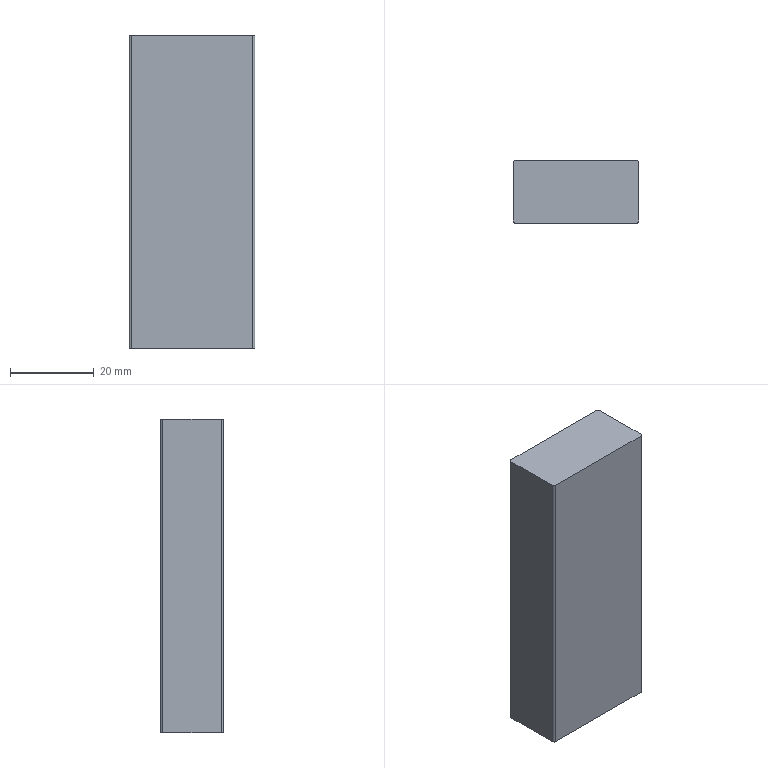Part | STEP file | 1 solid | 13 faces | box 30 x 15 x 75 mm | volume 33035 mm3 | plane 6 | cylinder 5 | cone 2 | commonest cylinder face diameters 1 x4 5 x1
STEP:
#1=CARTESIAN_POINT('',(0.,0.,0.));
#2=DIRECTION('',(0.,0.,1.));
#3=DIRECTION('',(1.,0.,0.));
#4=AXIS2_PLACEMENT_3D('',#1,#2,#3);
#5=CARTESIAN_POINT('',(1735.957,351.98,-43.381));
#6=VERTEX_POINT('',#5);
#7=CARTESIAN_POINT('',(1735.957,337.98,-43.381));
#8=VERTEX_POINT('',#7);
#9=CARTESIAN_POINT('',(1735.957,351.98,-43.381));
#10=DIRECTION('',(0.,-1.,0.));
#11=VECTOR('',#10,1.);
#12=LINE('',#9,#11);
#13=CARTESIAN_POINT('',(1735.957,351.98,33.675));
#14=DIRECTION('',(-1.,0.,0.));
#15=DIRECTION('',(0.,-1.,0.));
#16=AXIS2_PLACEMENT_3D('',#13,#14,#15);
#17=PLANE('',#16);
#18=CARTESIAN_POINT('',(0.,-77.056));
#19=DIRECTION('',(1.,0.));
#20=VECTOR('',#19,1.);
#21=LINE('',#18,#20);
#22=(GEOMETRIC_REPRESENTATION_CONTEXT(2)PARAMETRIC_REPRESENTATION_CONTEXT()REPRESENTATION_CONTEXT('',''));
#23=DEFINITIONAL_REPRESENTATION('',(#21),#22);
#24=PCURVE('',#17,#23);
#25=CARTESIAN_POINT('',(1735.457,337.98,-43.381));
#26=DIRECTION('',(0.,0.,1.));
#27=DIRECTION('',(-1.,0.,0.));
#28=AXIS2_PLACEMENT_3D('',#25,#26,#27);
#29=PLANE('',#28);
#30=CARTESIAN_POINT('',(-0.5,-14.));
#31=DIRECTION('',(0.,1.));
#32=VECTOR('',#31,1.);
#33=LINE('',#30,#32);
#34=(GEOMETRIC_REPRESENTATION_CONTEXT(2)PARAMETRIC_REPRESENTATION_CONTEXT()REPRESENTATION_CONTEXT('',''));
#35=DEFINITIONAL_REPRESENTATION('',(#33),#34);
#36=PCURVE('',#29,#35);
#37=SURFACE_CURVE('',#12,(#24,#36),.PCURVE_S1.);
#38=EDGE_CURVE('',#6,#8,#37,.T.);
#39=ORIENTED_EDGE('',*,*,#38,.F.);
#40=CARTESIAN_POINT('',(1735.957,351.98,31.619));
#41=VERTEX_POINT('',#40);
#42=CARTESIAN_POINT('',(1735.957,351.98,33.675));
#43=DIRECTION('',(0.,0.,-1.));
#44=VECTOR('',#43,1.);
#45=LINE('',#42,#44);
#46=CARTESIAN_POINT('',(0.,0.));
#47=DIRECTION('',(0.,-1.));
#48=VECTOR('',#47,1.);
#49=LINE('',#46,#48);
#50=(GEOMETRIC_REPRESENTATION_CONTEXT(2)PARAMETRIC_REPRESENTATION_CONTEXT()REPRESENTATION_CONTEXT('',''));
#51=DEFINITIONAL_REPRESENTATION('',(#49),#50);
#52=PCURVE('',#17,#51);
#53=CARTESIAN_POINT('',(1735.457,351.98,33.675));
#54=DIRECTION('',(0.,0.,-1.));
#55=DIRECTION('',(1.,0.,0.));
#56=AXIS2_PLACEMENT_3D('',#53,#54,#55);
#57=CYLINDRICAL_SURFACE('',#56,0.5);
#58=CARTESIAN_POINT('',(6.283,0.));
#59=DIRECTION('',(0.,1.));
#60=VECTOR('',#59,1.);
#61=LINE('',#58,#60);
#62=(GEOMETRIC_REPRESENTATION_CONTEXT(2)PARAMETRIC_REPRESENTATION_CONTEXT()REPRESENTATION_CONTEXT('',''));
#63=DEFINITIONAL_REPRESENTATION('',(#61),#62);
#64=PCURVE('',#57,#63);
#65=SURFACE_CURVE('',#45,(#52,#64),.PCURVE_S1.);
#66=EDGE_CURVE('',#41,#6,#65,.T.);
#67=ORIENTED_EDGE('',*,*,#66,.F.);
#68=CARTESIAN_POINT('',(1735.957,337.98,31.619));
#69=VERTEX_POINT('',#68);
#70=CARTESIAN_POINT('',(1735.957,337.98,31.619));
#71=DIRECTION('',(0.,-1.,0.));
#72=VECTOR('',#71,1.);
#73=LINE('',#70,#72);
#74=CARTESIAN_POINT('',(14.,-2.056));
#75=DIRECTION('',(1.,0.));
#76=VECTOR('',#75,1.);
#77=LINE('',#74,#76);
#78=(GEOMETRIC_REPRESENTATION_CONTEXT(2)PARAMETRIC_REPRESENTATION_CONTEXT()REPRESENTATION_CONTEXT('',''));
#79=DEFINITIONAL_REPRESENTATION('',(#77),#78);
#80=PCURVE('',#17,#79);
#81=CARTESIAN_POINT('',(1735.457,337.98,31.619));
#82=DIRECTION('',(0.,0.,1.));
#83=DIRECTION('',(-1.,0.,0.));
#84=AXIS2_PLACEMENT_3D('',#81,#82,#83);
#85=PLANE('',#84);
#86=CARTESIAN_POINT('',(-0.5,0.));
#87=DIRECTION('',(0.,1.));
#88=VECTOR('',#87,1.);
#89=LINE('',#86,#88);
#90=(GEOMETRIC_REPRESENTATION_CONTEXT(2)PARAMETRIC_REPRESENTATION_CONTEXT()REPRESENTATION_CONTEXT('',''));
#91=DEFINITIONAL_REPRESENTATION('',(#89),#90);
#92=PCURVE('',#85,#91);
#93=SURFACE_CURVE('',#73,(#80,#92),.PCURVE_S1.);
#94=EDGE_CURVE('',#41,#69,#93,.T.);
#95=ORIENTED_EDGE('',*,*,#94,.T.);
#96=CARTESIAN_POINT('',(1735.957,337.98,33.675));
#97=DIRECTION('',(0.,0.,-1.));
#98=VECTOR('',#97,1.);
#99=LINE('',#96,#98);
#100=CARTESIAN_POINT('',(14.,0.));
#101=DIRECTION('',(0.,-1.));
#102=VECTOR('',#101,1.);
#103=LINE('',#100,#102);
#104=(GEOMETRIC_REPRESENTATION_CONTEXT(2)PARAMETRIC_REPRESENTATION_CONTEXT()REPRESENTATION_CONTEXT('',''));
#105=DEFINITIONAL_REPRESENTATION('',(#103),#104);
#106=PCURVE('',#17,#105);
#107=CARTESIAN_POINT('',(1735.457,337.98,33.675));
#108=DIRECTION('',(0.,0.,-1.));
#109=DIRECTION('',(1.,0.,0.));
#110=AXIS2_PLACEMENT_3D('',#107,#108,#109);
#111=CYLINDRICAL_SURFACE('',#110,0.5);
#112=CARTESIAN_POINT('',(0.,0.));
#113=DIRECTION('',(0.,1.));
#114=VECTOR('',#113,1.);
#115=LINE('',#112,#114);
#116=(GEOMETRIC_REPRESENTATION_CONTEXT(2)PARAMETRIC_REPRESENTATION_CONTEXT()REPRESENTATION_CONTEXT('',''));
#117=DEFINITIONAL_REPRESENTATION('',(#115),#116);
#118=PCURVE('',#111,#117);
#119=SURFACE_CURVE('',#99,(#106,#118),.PCURVE_S1.);
#120=EDGE_CURVE('',#69,#8,#119,.T.);
#121=ORIENTED_EDGE('',*,*,#120,.T.);
#122=EDGE_LOOP('',(#39,#67,#95,#121));
#123=FACE_BOUND('',#122,.T.);
#124=ADVANCED_FACE('',(#123),#17,.F.);
#125=CARTESIAN_POINT('',(1735.457,337.48,-43.381));
#126=VERTEX_POINT('',#125);
#127=CARTESIAN_POINT('',(1735.457,337.98,-43.381));
#128=DIRECTION('',(0.,0.,-1.));
#129=DIRECTION('',(1.,0.,0.));
#130=AXIS2_PLACEMENT_3D('',#127,#128,#129);
#131=CIRCLE('',#130,0.5);
#132=CARTESIAN_POINT('',(0.,77.056));
#133=DIRECTION('',(1.,0.));
#134=VECTOR('',#133,1.);
#135=LINE('',#132,#134);
#136=(GEOMETRIC_REPRESENTATION_CONTEXT(2)PARAMETRIC_REPRESENTATION_CONTEXT()REPRESENTATION_CONTEXT('',''));
#137=DEFINITIONAL_REPRESENTATION('',(#135),#136);
#138=PCURVE('',#111,#137);
#139=CARTESIAN_POINT('',(-0.5,0.));
#140=CARTESIAN_POINT('',(-0.5,0.866));
#141=CARTESIAN_POINT('',(0.25,0.433));
#142=CARTESIAN_POINT('',(1.,0.));
#143=CARTESIAN_POINT('',(0.25,-0.433));
#144=CARTESIAN_POINT('',(-0.5,-0.866));
#145=CARTESIAN_POINT('',(-0.5,0.));
#146=(BOUNDED_CURVE()B_SPLINE_CURVE(2,(#139,#140,#141,#142,#143,#144,#145),.UNSPECIFIED.,.T.,.F.)B_SPLINE_CURVE_WITH_KNOTS((1,2,2,2,2,1),(-2.094,0.,2.094,4.189,6.283,8.378),.UNSPECIFIED.)CURVE()GEOMETRIC_REPRESENTATION_ITEM()RATIONAL_B_SPLINE_CURVE((1.,0.5,1.,0.5,1.,0.5,1.))REPRESENTATION_ITEM(''));
#147=(GEOMETRIC_REPRESENTATION_CONTEXT(2)PARAMETRIC_REPRESENTATION_CONTEXT()REPRESENTATION_CONTEXT('',''));
#148=DEFINITIONAL_REPRESENTATION('',(#146),#147);
#149=PCURVE('',#29,#148);
#150=SURFACE_CURVE('',#131,(#138,#149),.PCURVE_S1.);
#151=EDGE_CURVE('',#8,#126,#150,.T.);
#152=ORIENTED_EDGE('',*,*,#151,.F.);
#153=ORIENTED_EDGE('',*,*,#120,.F.);
#154=CARTESIAN_POINT('',(1735.457,337.48,31.619));
#155=VERTEX_POINT('',#154);
#156=CARTESIAN_POINT('',(1735.457,337.98,31.619));
#157=DIRECTION('',(0.,0.,-1.));
#158=DIRECTION('',(1.,0.,0.));
#159=AXIS2_PLACEMENT_3D('',#156,#157,#158);
#160=CIRCLE('',#159,0.5);
#161=CARTESIAN_POINT('',(0.,2.056));
#162=DIRECTION('',(1.,0.));
#163=VECTOR('',#162,1.);
#164=LINE('',#161,#163);
#165=(GEOMETRIC_REPRESENTATION_CONTEXT(2)PARAMETRIC_REPRESENTATION_CONTEXT()REPRESENTATION_CONTEXT('',''));
#166=DEFINITIONAL_REPRESENTATION('',(#164),#165);
#167=PCURVE('',#111,#166);
#168=CARTESIAN_POINT('',(-0.5,0.));
#169=CARTESIAN_POINT('',(-0.5,0.866));
#170=CARTESIAN_POINT('',(0.25,0.433));
#171=CARTESIAN_POINT('',(1.,0.));
#172=CARTESIAN_POINT('',(0.25,-0.433));
#173=CARTESIAN_POINT('',(-0.5,-0.866));
#174=CARTESIAN_POINT('',(-0.5,0.));
#175=(BOUNDED_CURVE()B_SPLINE_CURVE(2,(#168,#169,#170,#171,#172,#173,#174),.UNSPECIFIED.,.T.,.F.)B_SPLINE_CURVE_WITH_KNOTS((1,2,2,2,2,1),(-2.094,0.,2.094,4.189,6.283,8.378),.UNSPECIFIED.)CURVE()GEOMETRIC_REPRESENTATION_ITEM()RATIONAL_B_SPLINE_CURVE((1.,0.5,1.,0.5,1.,0.5,1.))REPRESENTATION_ITEM(''));
#176=(GEOMETRIC_REPRESENTATION_CONTEXT(2)PARAMETRIC_REPRESENTATION_CONTEXT()REPRESENTATION_CONTEXT('',''));
#177=DEFINITIONAL_REPRESENTATION('',(#175),#176);
#178=PCURVE('',#85,#177);
#179=SURFACE_CURVE('',#160,(#167,#178),.PCURVE_S1.);
#180=EDGE_CURVE('',#69,#155,#179,.T.);
#181=ORIENTED_EDGE('',*,*,#180,.T.);
#182=CARTESIAN_POINT('',(1735.457,337.48,33.675));
#183=DIRECTION('',(0.,0.,-1.));
#184=VECTOR('',#183,1.);
#185=LINE('',#182,#184);
#186=CARTESIAN_POINT('',(1.571,0.));
#187=DIRECTION('',(0.,1.));
#188=VECTOR('',#187,1.);
#189=LINE('',#186,#188);
#190=(GEOMETRIC_REPRESENTATION_CONTEXT(2)PARAMETRIC_REPRESENTATION_CONTEXT()REPRESENTATION_CONTEXT('',''));
#191=DEFINITIONAL_REPRESENTATION('',(#189),#190);
#192=PCURVE('',#111,#191);
#193=CARTESIAN_POINT('',(1735.457,337.48,33.675));
#194=DIRECTION('',(0.,1.,0.));
#195=DIRECTION('',(0.,0.,-1.));
#196=AXIS2_PLACEMENT_3D('',#193,#194,#195);
#197=PLANE('',#196);
#198=CARTESIAN_POINT('',(0.,0.));
#199=DIRECTION('',(1.,0.));
#200=VECTOR('',#199,1.);
#201=LINE('',#198,#200);
#202=(GEOMETRIC_REPRESENTATION_CONTEXT(2)PARAMETRIC_REPRESENTATION_CONTEXT()REPRESENTATION_CONTEXT('',''));
#203=DEFINITIONAL_REPRESENTATION('',(#201),#202);
#204=PCURVE('',#197,#203);
#205=SURFACE_CURVE('',#185,(#192,#204),.PCURVE_S1.);
#206=EDGE_CURVE('',#155,#126,#205,.T.);
#207=ORIENTED_EDGE('',*,*,#206,.T.);
#208=EDGE_LOOP('',(#152,#153,#181,#207));
#209=FACE_BOUND('',#208,.T.);
#210=ADVANCED_FACE('',(#209),#111,.T.);
#211=CARTESIAN_POINT('',(1706.457,337.48,-43.381));
#212=VERTEX_POINT('',#211);
#213=CARTESIAN_POINT('',(1735.457,337.48,-43.381));
#214=DIRECTION('',(-1.,0.,0.));
#215=VECTOR('',#214,1.);
#216=LINE('',#213,#215);
#217=CARTESIAN_POINT('',(77.056,0.));
#218=DIRECTION('',(0.,1.));
#219=VECTOR('',#218,1.);
#220=LINE('',#217,#219);
#221=(GEOMETRIC_REPRESENTATION_CONTEXT(2)PARAMETRIC_REPRESENTATION_CONTEXT()REPRESENTATION_CONTEXT('',''));
#222=DEFINITIONAL_REPRESENTATION('',(#220),#221);
#223=PCURVE('',#197,#222);
#224=CARTESIAN_POINT('',(0.,0.5));
#225=DIRECTION('',(1.,0.));
#226=VECTOR('',#225,1.);
#227=LINE('',#224,#226);
#228=(GEOMETRIC_REPRESENTATION_CONTEXT(2)PARAMETRIC_REPRESENTATION_CONTEXT()REPRESENTATION_CONTEXT('',''));
#229=DEFINITIONAL_REPRESENTATION('',(#227),#228);
#230=PCURVE('',#29,#229);
#231=SURFACE_CURVE('',#216,(#223,#230),.PCURVE_S1.);
#232=EDGE_CURVE('',#126,#212,#231,.T.);
#233=ORIENTED_EDGE('',*,*,#232,.F.);
#234=ORIENTED_EDGE('',*,*,#206,.F.);
#235=CARTESIAN_POINT('',(1706.457,337.48,31.619));
#236=VERTEX_POINT('',#235);
#237=CARTESIAN_POINT('',(1735.457,337.48,31.619));
#238=DIRECTION('',(-1.,0.,0.));
#239=VECTOR('',#238,1.);
#240=LINE('',#237,#239);
#241=CARTESIAN_POINT('',(2.056,0.));
#242=DIRECTION('',(0.,1.));
#243=VECTOR('',#242,1.);
#244=LINE('',#241,#243);
#245=(GEOMETRIC_REPRESENTATION_CONTEXT(2)PARAMETRIC_REPRESENTATION_CONTEXT()REPRESENTATION_CONTEXT('',''));
#246=DEFINITIONAL_REPRESENTATION('',(#244),#245);
#247=PCURVE('',#197,#246);
#248=CARTESIAN_POINT('',(0.,0.5));
#249=DIRECTION('',(1.,0.));
#250=VECTOR('',#249,1.);
#251=LINE('',#248,#250);
#252=(GEOMETRIC_REPRESENTATION_CONTEXT(2)PARAMETRIC_REPRESENTATION_CONTEXT()REPRESENTATION_CONTEXT('',''));
#253=DEFINITIONAL_REPRESENTATION('',(#251),#252);
#254=PCURVE('',#85,#253);
#255=SURFACE_CURVE('',#240,(#247,#254),.PCURVE_S1.);
#256=EDGE_CURVE('',#155,#236,#255,.T.);
#257=ORIENTED_EDGE('',*,*,#256,.T.);
#258=CARTESIAN_POINT('',(1706.457,337.48,33.675));
#259=DIRECTION('',(0.,0.,-1.));
#260=VECTOR('',#259,1.);
#261=LINE('',#258,#260);
#262=CARTESIAN_POINT('',(0.,29.));
#263=DIRECTION('',(1.,0.));
#264=VECTOR('',#263,1.);
#265=LINE('',#262,#264);
#266=(GEOMETRIC_REPRESENTATION_CONTEXT(2)PARAMETRIC_REPRESENTATION_CONTEXT()REPRESENTATION_CONTEXT('',''));
#267=DEFINITIONAL_REPRESENTATION('',(#265),#266);
#268=PCURVE('',#197,#267);
#269=CARTESIAN_POINT('',(1706.457,337.98,33.675));
#270=DIRECTION('',(0.,0.,-1.));
#271=DIRECTION('',(1.,0.,0.));
#272=AXIS2_PLACEMENT_3D('',#269,#270,#271);
#273=CYLINDRICAL_SURFACE('',#272,0.5);
#274=CARTESIAN_POINT('',(1.571,0.));
#275=DIRECTION('',(0.,1.));
#276=VECTOR('',#275,1.);
#277=LINE('',#274,#276);
#278=(GEOMETRIC_REPRESENTATION_CONTEXT(2)PARAMETRIC_REPRESENTATION_CONTEXT()REPRESENTATION_CONTEXT('',''));
#279=DEFINITIONAL_REPRESENTATION('',(#277),#278);
#280=PCURVE('',#273,#279);
#281=SURFACE_CURVE('',#261,(#268,#280),.PCURVE_S1.);
#282=EDGE_CURVE('',#236,#212,#281,.T.);
#283=ORIENTED_EDGE('',*,*,#282,.T.);
#284=EDGE_LOOP('',(#233,#234,#257,#283));
#285=FACE_BOUND('',#284,.T.);
#286=ADVANCED_FACE('',(#285),#197,.F.);
#287=CARTESIAN_POINT('',(1705.957,337.98,-43.381));
#288=VERTEX_POINT('',#287);
#289=CARTESIAN_POINT('',(1706.457,337.98,-43.381));
#290=DIRECTION('',(0.,0.,-1.));
#291=DIRECTION('',(1.,0.,0.));
#292=AXIS2_PLACEMENT_3D('',#289,#290,#291);
#293=CIRCLE('',#292,0.5);
#294=CARTESIAN_POINT('',(0.,77.056));
#295=DIRECTION('',(1.,0.));
#296=VECTOR('',#295,1.);
#297=LINE('',#294,#296);
#298=(GEOMETRIC_REPRESENTATION_CONTEXT(2)PARAMETRIC_REPRESENTATION_CONTEXT()REPRESENTATION_CONTEXT('',''));
#299=DEFINITIONAL_REPRESENTATION('',(#297),#298);
#300=PCURVE('',#273,#299);
#301=CARTESIAN_POINT('',(28.5,0.));
#302=CARTESIAN_POINT('',(28.5,0.866));
#303=CARTESIAN_POINT('',(29.25,0.433));
#304=CARTESIAN_POINT('',(30.,0.));
#305=CARTESIAN_POINT('',(29.25,-0.433));
#306=CARTESIAN_POINT('',(28.5,-0.866));
#307=CARTESIAN_POINT('',(28.5,0.));
#308=(BOUNDED_CURVE()B_SPLINE_CURVE(2,(#301,#302,#303,#304,#305,#306,#307),.UNSPECIFIED.,.T.,.F.)B_SPLINE_CURVE_WITH_KNOTS((1,2,2,2,2,1),(-2.094,0.,2.094,4.189,6.283,8.378),.UNSPECIFIED.)CURVE()GEOMETRIC_REPRESENTATION_ITEM()RATIONAL_B_SPLINE_CURVE((1.,0.5,1.,0.5,1.,0.5,1.))REPRESENTATION_ITEM(''));
#309=(GEOMETRIC_REPRESENTATION_CONTEXT(2)PARAMETRIC_REPRESENTATION_CONTEXT()REPRESENTATION_CONTEXT('',''));
#310=DEFINITIONAL_REPRESENTATION('',(#308),#309);
#311=PCURVE('',#29,#310);
#312=SURFACE_CURVE('',#293,(#300,#311),.PCURVE_S1.);
#313=EDGE_CURVE('',#212,#288,#312,.T.);
#314=ORIENTED_EDGE('',*,*,#313,.F.);
#315=ORIENTED_EDGE('',*,*,#282,.F.);
#316=CARTESIAN_POINT('',(1705.957,337.98,31.619));
#317=VERTEX_POINT('',#316);
#318=CARTESIAN_POINT('',(1706.457,337.98,31.619));
#319=DIRECTION('',(0.,0.,-1.));
#320=DIRECTION('',(1.,0.,0.));
#321=AXIS2_PLACEMENT_3D('',#318,#319,#320);
#322=CIRCLE('',#321,0.5);
#323=CARTESIAN_POINT('',(0.,2.056));
#324=DIRECTION('',(1.,0.));
#325=VECTOR('',#324,1.);
#326=LINE('',#323,#325);
#327=(GEOMETRIC_REPRESENTATION_CONTEXT(2)PARAMETRIC_REPRESENTATION_CONTEXT()REPRESENTATION_CONTEXT('',''));
#328=DEFINITIONAL_REPRESENTATION('',(#326),#327);
#329=PCURVE('',#273,#328);
#330=CARTESIAN_POINT('',(28.5,0.));
#331=CARTESIAN_POINT('',(28.5,0.866));
#332=CARTESIAN_POINT('',(29.25,0.433));
#333=CARTESIAN_POINT('',(30.,0.));
#334=CARTESIAN_POINT('',(29.25,-0.433));
#335=CARTESIAN_POINT('',(28.5,-0.866));
#336=CARTESIAN_POINT('',(28.5,0.));
#337=(BOUNDED_CURVE()B_SPLINE_CURVE(2,(#330,#331,#332,#333,#334,#335,#336),.UNSPECIFIED.,.T.,.F.)B_SPLINE_CURVE_WITH_KNOTS((1,2,2,2,2,1),(-2.094,0.,2.094,4.189,6.283,8.378),.UNSPECIFIED.)CURVE()GEOMETRIC_REPRESENTATION_ITEM()RATIONAL_B_SPLINE_CURVE((1.,0.5,1.,0.5,1.,0.5,1.))REPRESENTATION_ITEM(''));
#338=(GEOMETRIC_REPRESENTATION_CONTEXT(2)PARAMETRIC_REPRESENTATION_CONTEXT()REPRESENTATION_CONTEXT('',''));
#339=DEFINITIONAL_REPRESENTATION('',(#337),#338);
#340=PCURVE('',#85,#339);
#341=SURFACE_CURVE('',#322,(#329,#340),.PCURVE_S1.);
#342=EDGE_CURVE('',#236,#317,#341,.T.);
#343=ORIENTED_EDGE('',*,*,#342,.T.);
#344=CARTESIAN_POINT('',(1705.957,337.98,33.675));
#345=DIRECTION('',(0.,0.,-1.));
#346=VECTOR('',#345,1.);
#347=LINE('',#344,#346);
#348=CARTESIAN_POINT('',(3.142,0.));
#349=DIRECTION('',(0.,1.));
#350=VECTOR('',#349,1.);
#351=LINE('',#348,#350);
#352=(GEOMETRIC_REPRESENTATION_CONTEXT(2)PARAMETRIC_REPRESENTATION_CONTEXT()REPRESENTATION_CONTEXT('',''));
#353=DEFINITIONAL_REPRESENTATION('',(#351),#352);
#354=PCURVE('',#273,#353);
#355=CARTESIAN_POINT('',(1705.957,337.98,33.675));
#356=DIRECTION('',(1.,0.,0.));
#357=DIRECTION('',(0.,0.,1.));
#358=AXIS2_PLACEMENT_3D('',#355,#356,#357);
#359=PLANE('',#358);
#360=CARTESIAN_POINT('',(0.,0.));
#361=DIRECTION('',(-1.,0.));
#362=VECTOR('',#361,1.);
#363=LINE('',#360,#362);
#364=(GEOMETRIC_REPRESENTATION_CONTEXT(2)PARAMETRIC_REPRESENTATION_CONTEXT()REPRESENTATION_CONTEXT('',''));
#365=DEFINITIONAL_REPRESENTATION('',(#363),#364);
#366=PCURVE('',#359,#365);
#367=SURFACE_CURVE('',#347,(#354,#366),.PCURVE_S1.);
#368=EDGE_CURVE('',#317,#288,#367,.T.);
#369=ORIENTED_EDGE('',*,*,#368,.T.);
#370=EDGE_LOOP('',(#314,#315,#343,#369));
#371=FACE_BOUND('',#370,.T.);
#372=ADVANCED_FACE('',(#371),#273,.T.);
#373=CARTESIAN_POINT('',(1705.957,351.98,-43.381));
#374=VERTEX_POINT('',#373);
#375=CARTESIAN_POINT('',(1705.957,337.98,-43.381));
#376=DIRECTION('',(0.,1.,0.));
#377=VECTOR('',#376,1.);
#378=LINE('',#375,#377);
#379=CARTESIAN_POINT('',(-77.056,0.));
#380=DIRECTION('',(0.,-1.));
#381=VECTOR('',#380,1.);
#382=LINE('',#379,#381);
#383=(GEOMETRIC_REPRESENTATION_CONTEXT(2)PARAMETRIC_REPRESENTATION_CONTEXT()REPRESENTATION_CONTEXT('',''));
#384=DEFINITIONAL_REPRESENTATION('',(#382),#383);
#385=PCURVE('',#359,#384);
#386=CARTESIAN_POINT('',(29.5,0.));
#387=DIRECTION('',(0.,-1.));
#388=VECTOR('',#387,1.);
#389=LINE('',#386,#388);
#390=(GEOMETRIC_REPRESENTATION_CONTEXT(2)PARAMETRIC_REPRESENTATION_CONTEXT()REPRESENTATION_CONTEXT('',''));
#391=DEFINITIONAL_REPRESENTATION('',(#389),#390);
#392=PCURVE('',#29,#391);
#393=SURFACE_CURVE('',#378,(#385,#392),.PCURVE_S1.);
#394=EDGE_CURVE('',#288,#374,#393,.T.);
#395=ORIENTED_EDGE('',*,*,#394,.F.);
#396=ORIENTED_EDGE('',*,*,#368,.F.);
#397=CARTESIAN_POINT('',(1705.957,351.98,31.619));
#398=VERTEX_POINT('',#397);
#399=CARTESIAN_POINT('',(1705.957,337.98,31.619));
#400=DIRECTION('',(0.,1.,0.));
#401=VECTOR('',#400,1.);
#402=LINE('',#399,#401);
#403=CARTESIAN_POINT('',(-2.056,0.));
#404=DIRECTION('',(0.,-1.));
#405=VECTOR('',#404,1.);
#406=LINE('',#403,#405);
#407=(GEOMETRIC_REPRESENTATION_CONTEXT(2)PARAMETRIC_REPRESENTATION_CONTEXT()REPRESENTATION_CONTEXT('',''));
#408=DEFINITIONAL_REPRESENTATION('',(#406),#407);
#409=PCURVE('',#359,#408);
#410=CARTESIAN_POINT('',(29.5,0.));
#411=DIRECTION('',(0.,-1.));
#412=VECTOR('',#411,1.);
#413=LINE('',#410,#412);
#414=(GEOMETRIC_REPRESENTATION_CONTEXT(2)PARAMETRIC_REPRESENTATION_CONTEXT()REPRESENTATION_CONTEXT('',''));
#415=DEFINITIONAL_REPRESENTATION('',(#413),#414);
#416=PCURVE('',#85,#415);
#417=SURFACE_CURVE('',#402,(#409,#416),.PCURVE_S1.);
#418=EDGE_CURVE('',#317,#398,#417,.T.);
#419=ORIENTED_EDGE('',*,*,#418,.T.);
#420=CARTESIAN_POINT('',(1705.957,351.98,33.675));
#421=DIRECTION('',(0.,0.,-1.));
#422=VECTOR('',#421,1.);
#423=LINE('',#420,#422);
#424=CARTESIAN_POINT('',(0.,-14.));
#425=DIRECTION('',(-1.,0.));
#426=VECTOR('',#425,1.);
#427=LINE('',#424,#426);
#428=(GEOMETRIC_REPRESENTATION_CONTEXT(2)PARAMETRIC_REPRESENTATION_CONTEXT()REPRESENTATION_CONTEXT('',''));
#429=DEFINITIONAL_REPRESENTATION('',(#427),#428);
#430=PCURVE('',#359,#429);
#431=CARTESIAN_POINT('',(1706.457,351.98,33.675));
#432=DIRECTION('',(0.,0.,-1.));
#433=DIRECTION('',(1.,0.,0.));
#434=AXIS2_PLACEMENT_3D('',#431,#432,#433);
#435=CYLINDRICAL_SURFACE('',#434,0.5);
#436=CARTESIAN_POINT('',(3.142,0.));
#437=DIRECTION('',(0.,1.));
#438=VECTOR('',#437,1.);
#439=LINE('',#436,#438);
#440=(GEOMETRIC_REPRESENTATION_CONTEXT(2)PARAMETRIC_REPRESENTATION_CONTEXT()REPRESENTATION_CONTEXT('',''));
#441=DEFINITIONAL_REPRESENTATION('',(#439),#440);
#442=PCURVE('',#435,#441);
#443=SURFACE_CURVE('',#423,(#430,#442),.PCURVE_S1.);
#444=EDGE_CURVE('',#398,#374,#443,.T.);
#445=ORIENTED_EDGE('',*,*,#444,.T.);
#446=EDGE_LOOP('',(#395,#396,#419,#445));
#447=FACE_BOUND('',#446,.T.);
#448=ADVANCED_FACE('',(#447),#359,.F.);
#449=CARTESIAN_POINT('',(1706.457,352.48,-43.381));
#450=VERTEX_POINT('',#449);
#451=CARTESIAN_POINT('',(1706.457,351.98,-43.381));
#452=DIRECTION('',(0.,0.,-1.));
#453=DIRECTION('',(1.,0.,0.));
#454=AXIS2_PLACEMENT_3D('',#451,#452,#453);
#455=CIRCLE('',#454,0.5);
#456=CARTESIAN_POINT('',(0.,77.056));
#457=DIRECTION('',(1.,0.));
#458=VECTOR('',#457,1.);
#459=LINE('',#456,#458);
#460=(GEOMETRIC_REPRESENTATION_CONTEXT(2)PARAMETRIC_REPRESENTATION_CONTEXT()REPRESENTATION_CONTEXT('',''));
#461=DEFINITIONAL_REPRESENTATION('',(#459),#460);
#462=PCURVE('',#435,#461);
#463=CARTESIAN_POINT('',(28.5,-14.));
#464=CARTESIAN_POINT('',(28.5,-13.134));
#465=CARTESIAN_POINT('',(29.25,-13.567));
#466=CARTESIAN_POINT('',(30.,-14.));
#467=CARTESIAN_POINT('',(29.25,-14.433));
#468=CARTESIAN_POINT('',(28.5,-14.866));
#469=CARTESIAN_POINT('',(28.5,-14.));
#470=(BOUNDED_CURVE()B_SPLINE_CURVE(2,(#463,#464,#465,#466,#467,#468,#469),.UNSPECIFIED.,.T.,.F.)B_SPLINE_CURVE_WITH_KNOTS((1,2,2,2,2,1),(-2.094,0.,2.094,4.189,6.283,8.378),.UNSPECIFIED.)CURVE()GEOMETRIC_REPRESENTATION_ITEM()RATIONAL_B_SPLINE_CURVE((1.,0.5,1.,0.5,1.,0.5,1.))REPRESENTATION_ITEM(''));
#471=(GEOMETRIC_REPRESENTATION_CONTEXT(2)PARAMETRIC_REPRESENTATION_CONTEXT()REPRESENTATION_CONTEXT('',''));
#472=DEFINITIONAL_REPRESENTATION('',(#470),#471);
#473=PCURVE('',#29,#472);
#474=SURFACE_CURVE('',#455,(#462,#473),.PCURVE_S1.);
#475=EDGE_CURVE('',#374,#450,#474,.T.);
#476=ORIENTED_EDGE('',*,*,#475,.F.);
#477=ORIENTED_EDGE('',*,*,#444,.F.);
#478=CARTESIAN_POINT('',(1706.457,352.48,31.619));
#479=VERTEX_POINT('',#478);
#480=CARTESIAN_POINT('',(1706.457,351.98,31.619));
#481=DIRECTION('',(0.,0.,-1.));
#482=DIRECTION('',(1.,0.,0.));
#483=AXIS2_PLACEMENT_3D('',#480,#481,#482);
#484=CIRCLE('',#483,0.5);
#485=CARTESIAN_POINT('',(0.,2.056));
#486=DIRECTION('',(1.,0.));
#487=VECTOR('',#486,1.);
#488=LINE('',#485,#487);
#489=(GEOMETRIC_REPRESENTATION_CONTEXT(2)PARAMETRIC_REPRESENTATION_CONTEXT()REPRESENTATION_CONTEXT('',''));
#490=DEFINITIONAL_REPRESENTATION('',(#488),#489);
#491=PCURVE('',#435,#490);
#492=CARTESIAN_POINT('',(28.5,-14.));
#493=CARTESIAN_POINT('',(28.5,-13.134));
#494=CARTESIAN_POINT('',(29.25,-13.567));
#495=CARTESIAN_POINT('',(30.,-14.));
#496=CARTESIAN_POINT('',(29.25,-14.433));
#497=CARTESIAN_POINT('',(28.5,-14.866));
#498=CARTESIAN_POINT('',(28.5,-14.));
#499=(BOUNDED_CURVE()B_SPLINE_CURVE(2,(#492,#493,#494,#495,#496,#497,#498),.UNSPECIFIED.,.T.,.F.)B_SPLINE_CURVE_WITH_KNOTS((1,2,2,2,2,1),(-2.094,0.,2.094,4.189,6.283,8.378),.UNSPECIFIED.)CURVE()GEOMETRIC_REPRESENTATION_ITEM()RATIONAL_B_SPLINE_CURVE((1.,0.5,1.,0.5,1.,0.5,1.))REPRESENTATION_ITEM(''));
#500=(GEOMETRIC_REPRESENTATION_CONTEXT(2)PARAMETRIC_REPRESENTATION_CONTEXT()REPRESENTATION_CONTEXT('',''));
#501=DEFINITIONAL_REPRESENTATION('',(#499),#500);
#502=PCURVE('',#85,#501);
#503=SURFACE_CURVE('',#484,(#491,#502),.PCURVE_S1.);
#504=EDGE_CURVE('',#398,#479,#503,.T.);
#505=ORIENTED_EDGE('',*,*,#504,.T.);
#506=CARTESIAN_POINT('',(1706.457,352.48,33.675));
#507=DIRECTION('',(0.,0.,-1.));
#508=VECTOR('',#507,1.);
#509=LINE('',#506,#508);
#510=CARTESIAN_POINT('',(4.712,0.));
#511=DIRECTION('',(0.,1.));
#512=VECTOR('',#511,1.);
#513=LINE('',#510,#512);
#514=(GEOMETRIC_REPRESENTATION_CONTEXT(2)PARAMETRIC_REPRESENTATION_CONTEXT()REPRESENTATION_CONTEXT('',''));
#515=DEFINITIONAL_REPRESENTATION('',(#513),#514);
#516=PCURVE('',#435,#515);
#517=CARTESIAN_POINT('',(1706.457,352.48,33.675));
#518=DIRECTION('',(0.,-1.,0.));
#519=DIRECTION('',(0.,0.,1.));
#520=AXIS2_PLACEMENT_3D('',#517,#518,#519);
#521=PLANE('',#520);
#522=CARTESIAN_POINT('',(0.,0.));
#523=DIRECTION('',(-1.,0.));
#524=VECTOR('',#523,1.);
#525=LINE('',#522,#524);
#526=(GEOMETRIC_REPRESENTATION_CONTEXT(2)PARAMETRIC_REPRESENTATION_CONTEXT()REPRESENTATION_CONTEXT('',''));
#527=DEFINITIONAL_REPRESENTATION('',(#525),#526);
#528=PCURVE('',#521,#527);
#529=SURFACE_CURVE('',#509,(#516,#528),.PCURVE_S1.);
#530=EDGE_CURVE('',#479,#450,#529,.T.);
#531=ORIENTED_EDGE('',*,*,#530,.T.);
#532=EDGE_LOOP('',(#476,#477,#505,#531));
#533=FACE_BOUND('',#532,.T.);
#534=ADVANCED_FACE('',(#533),#435,.T.);
#535=CARTESIAN_POINT('',(1735.457,352.48,-43.381));
#536=VERTEX_POINT('',#535);
#537=CARTESIAN_POINT('',(1706.457,352.48,-43.381));
#538=DIRECTION('',(1.,0.,0.));
#539=VECTOR('',#538,1.);
#540=LINE('',#537,#539);
#541=CARTESIAN_POINT('',(-77.056,0.));
#542=DIRECTION('',(0.,-1.));
#543=VECTOR('',#542,1.);
#544=LINE('',#541,#543);
#545=(GEOMETRIC_REPRESENTATION_CONTEXT(2)PARAMETRIC_REPRESENTATION_CONTEXT()REPRESENTATION_CONTEXT('',''));
#546=DEFINITIONAL_REPRESENTATION('',(#544),#545);
#547=PCURVE('',#521,#546);
#548=CARTESIAN_POINT('',(29.,-14.5));
#549=DIRECTION('',(-1.,0.));
#550=VECTOR('',#549,1.);
#551=LINE('',#548,#550);
#552=(GEOMETRIC_REPRESENTATION_CONTEXT(2)PARAMETRIC_REPRESENTATION_CONTEXT()REPRESENTATION_CONTEXT('',''));
#553=DEFINITIONAL_REPRESENTATION('',(#551),#552);
#554=PCURVE('',#29,#553);
#555=SURFACE_CURVE('',#540,(#547,#554),.PCURVE_S1.);
#556=EDGE_CURVE('',#450,#536,#555,.T.);
#557=ORIENTED_EDGE('',*,*,#556,.F.);
#558=ORIENTED_EDGE('',*,*,#530,.F.);
#559=CARTESIAN_POINT('',(1735.457,352.48,31.619));
#560=VERTEX_POINT('',#559);
#561=CARTESIAN_POINT('',(1735.457,352.48,31.619));
#562=DIRECTION('',(1.,0.,0.));
#563=VECTOR('',#562,1.);
#564=LINE('',#561,#563);
#565=CARTESIAN_POINT('',(-2.056,-29.));
#566=DIRECTION('',(0.,-1.));
#567=VECTOR('',#566,1.);
#568=LINE('',#565,#567);
#569=(GEOMETRIC_REPRESENTATION_CONTEXT(2)PARAMETRIC_REPRESENTATION_CONTEXT()REPRESENTATION_CONTEXT('',''));
#570=DEFINITIONAL_REPRESENTATION('',(#568),#569);
#571=PCURVE('',#521,#570);
#572=CARTESIAN_POINT('',(0.,-14.5));
#573=DIRECTION('',(-1.,0.));
#574=VECTOR('',#573,1.);
#575=LINE('',#572,#574);
#576=(GEOMETRIC_REPRESENTATION_CONTEXT(2)PARAMETRIC_REPRESENTATION_CONTEXT()REPRESENTATION_CONTEXT('',''));
#577=DEFINITIONAL_REPRESENTATION('',(#575),#576);
#578=PCURVE('',#85,#577);
#579=SURFACE_CURVE('',#564,(#571,#578),.PCURVE_S1.);
#580=EDGE_CURVE('',#479,#560,#579,.T.);
#581=ORIENTED_EDGE('',*,*,#580,.T.);
#582=CARTESIAN_POINT('',(1735.457,352.48,33.675));
#583=DIRECTION('',(0.,0.,-1.));
#584=VECTOR('',#583,1.);
#585=LINE('',#582,#584);
#586=CARTESIAN_POINT('',(0.,-29.));
#587=DIRECTION('',(-1.,0.));
#588=VECTOR('',#587,1.);
#589=LINE('',#586,#588);
#590=(GEOMETRIC_REPRESENTATION_CONTEXT(2)PARAMETRIC_REPRESENTATION_CONTEXT()REPRESENTATION_CONTEXT('',''));
#591=DEFINITIONAL_REPRESENTATION('',(#589),#590);
#592=PCURVE('',#521,#591);
#593=CARTESIAN_POINT('',(4.712,0.));
#594=DIRECTION('',(0.,1.));
#595=VECTOR('',#594,1.);
#596=LINE('',#593,#595);
#597=(GEOMETRIC_REPRESENTATION_CONTEXT(2)PARAMETRIC_REPRESENTATION_CONTEXT()REPRESENTATION_CONTEXT('',''));
#598=DEFINITIONAL_REPRESENTATION('',(#596),#597);
#599=PCURVE('',#57,#598);
#600=SURFACE_CURVE('',#585,(#592,#599),.PCURVE_S1.);
#601=EDGE_CURVE('',#560,#536,#600,.T.);
#602=ORIENTED_EDGE('',*,*,#601,.T.);
#603=EDGE_LOOP('',(#557,#558,#581,#602));
#604=FACE_BOUND('',#603,.T.);
#605=ADVANCED_FACE('',(#604),#521,.F.);
#606=CARTESIAN_POINT('',(1735.457,351.98,-43.381));
#607=DIRECTION('',(0.,0.,-1.));
#608=DIRECTION('',(1.,0.,0.));
#609=AXIS2_PLACEMENT_3D('',#606,#607,#608);
#610=CIRCLE('',#609,0.5);
#611=CARTESIAN_POINT('',(0.,77.056));
#612=DIRECTION('',(1.,0.));
#613=VECTOR('',#612,1.);
#614=LINE('',#611,#613);
#615=(GEOMETRIC_REPRESENTATION_CONTEXT(2)PARAMETRIC_REPRESENTATION_CONTEXT()REPRESENTATION_CONTEXT('',''));
#616=DEFINITIONAL_REPRESENTATION('',(#614),#615);
#617=PCURVE('',#57,#616);
#618=CARTESIAN_POINT('',(-0.5,-14.));
#619=CARTESIAN_POINT('',(-0.5,-13.134));
#620=CARTESIAN_POINT('',(0.25,-13.567));
#621=CARTESIAN_POINT('',(1.,-14.));
#622=CARTESIAN_POINT('',(0.25,-14.433));
#623=CARTESIAN_POINT('',(-0.5,-14.866));
#624=CARTESIAN_POINT('',(-0.5,-14.));
#625=(BOUNDED_CURVE()B_SPLINE_CURVE(2,(#618,#619,#620,#621,#622,#623,#624),.UNSPECIFIED.,.T.,.F.)B_SPLINE_CURVE_WITH_KNOTS((1,2,2,2,2,1),(-2.094,0.,2.094,4.189,6.283,8.378),.UNSPECIFIED.)CURVE()GEOMETRIC_REPRESENTATION_ITEM()RATIONAL_B_SPLINE_CURVE((1.,0.5,1.,0.5,1.,0.5,1.))REPRESENTATION_ITEM(''));
#626=(GEOMETRIC_REPRESENTATION_CONTEXT(2)PARAMETRIC_REPRESENTATION_CONTEXT()REPRESENTATION_CONTEXT('',''));
#627=DEFINITIONAL_REPRESENTATION('',(#625),#626);
#628=PCURVE('',#29,#627);
#629=SURFACE_CURVE('',#610,(#617,#628),.PCURVE_S1.);
#630=EDGE_CURVE('',#536,#6,#629,.T.);
#631=ORIENTED_EDGE('',*,*,#630,.F.);
#632=ORIENTED_EDGE('',*,*,#601,.F.);
#633=CARTESIAN_POINT('',(1735.457,351.98,31.619));
#634=DIRECTION('',(0.,0.,-1.));
#635=DIRECTION('',(1.,0.,0.));
#636=AXIS2_PLACEMENT_3D('',#633,#634,#635);
#637=CIRCLE('',#636,0.5);
#638=CARTESIAN_POINT('',(0.,2.056));
#639=DIRECTION('',(1.,0.));
#640=VECTOR('',#639,1.);
#641=LINE('',#638,#640);
#642=(GEOMETRIC_REPRESENTATION_CONTEXT(2)PARAMETRIC_REPRESENTATION_CONTEXT()REPRESENTATION_CONTEXT('',''));
#643=DEFINITIONAL_REPRESENTATION('',(#641),#642);
#644=PCURVE('',#57,#643);
#645=CARTESIAN_POINT('',(-0.5,-14.));
#646=CARTESIAN_POINT('',(-0.5,-13.134));
#647=CARTESIAN_POINT('',(0.25,-13.567));
#648=CARTESIAN_POINT('',(1.,-14.));
#649=CARTESIAN_POINT('',(0.25,-14.433));
#650=CARTESIAN_POINT('',(-0.5,-14.866));
#651=CARTESIAN_POINT('',(-0.5,-14.));
#652=(BOUNDED_CURVE()B_SPLINE_CURVE(2,(#645,#646,#647,#648,#649,#650,#651),.UNSPECIFIED.,.T.,.F.)B_SPLINE_CURVE_WITH_KNOTS((1,2,2,2,2,1),(-2.094,0.,2.094,4.189,6.283,8.378),.UNSPECIFIED.)CURVE()GEOMETRIC_REPRESENTATION_ITEM()RATIONAL_B_SPLINE_CURVE((1.,0.5,1.,0.5,1.,0.5,1.))REPRESENTATION_ITEM(''));
#653=(GEOMETRIC_REPRESENTATION_CONTEXT(2)PARAMETRIC_REPRESENTATION_CONTEXT()REPRESENTATION_CONTEXT('',''));
#654=DEFINITIONAL_REPRESENTATION('',(#652),#653);
#655=PCURVE('',#85,#654);
#656=SURFACE_CURVE('',#637,(#644,#655),.PCURVE_S1.);
#657=EDGE_CURVE('',#560,#41,#656,.T.);
#658=ORIENTED_EDGE('',*,*,#657,.T.);
#659=ORIENTED_EDGE('',*,*,#66,.T.);
#660=EDGE_LOOP('',(#631,#632,#658,#659));
#661=FACE_BOUND('',#660,.T.);
#662=ADVANCED_FACE('',(#661),#57,.T.);
#663=ORIENTED_EDGE('',*,*,#94,.F.);
#664=ORIENTED_EDGE('',*,*,#657,.F.);
#665=ORIENTED_EDGE('',*,*,#580,.F.);
#666=ORIENTED_EDGE('',*,*,#504,.F.);
#667=ORIENTED_EDGE('',*,*,#418,.F.);
#668=ORIENTED_EDGE('',*,*,#342,.F.);
#669=ORIENTED_EDGE('',*,*,#256,.F.);
#670=ORIENTED_EDGE('',*,*,#180,.F.);
#671=EDGE_LOOP('',(#663,#664,#665,#666,#667,#668,#669,#670));
#672=FACE_BOUND('',#671,.T.);
#673=ADVANCED_FACE('',(#672),#85,.T.);
#674=CARTESIAN_POINT('',(1717.957,344.98,-43.381));
#675=VERTEX_POINT('',#674);
#676=CARTESIAN_POINT('',(1720.957,344.98,-43.381));
#677=DIRECTION('',(0.,0.,1.));
#678=DIRECTION('',(-1.,0.,0.));
#679=AXIS2_PLACEMENT_3D('',#676,#677,#678);
#680=CIRCLE('',#679,3.);
#681=CARTESIAN_POINT('',(14.5,-7.));
#682=DIRECTION('',(1.,0.));
#683=AXIS2_PLACEMENT_2D('',#681,#682);
#684=CIRCLE('',#683,3.);
#685=(GEOMETRIC_REPRESENTATION_CONTEXT(2)PARAMETRIC_REPRESENTATION_CONTEXT()REPRESENTATION_CONTEXT('',''));
#686=DEFINITIONAL_REPRESENTATION('',(#684),#685);
#687=PCURVE('',#29,#686);
#688=CARTESIAN_POINT('',(1720.957,344.98,-43.381));
#689=DIRECTION('',(0.,0.,-1.));
#690=DIRECTION('',(1.,0.,0.));
#691=AXIS2_PLACEMENT_3D('',#688,#689,#690);
#692=CONICAL_SURFACE('',#691,3.,0.7854);
#693=CARTESIAN_POINT('',(9.425,0.));
#694=DIRECTION('',(-1.,0.));
#695=VECTOR('',#694,1.);
#696=LINE('',#693,#695);
#697=(GEOMETRIC_REPRESENTATION_CONTEXT(2)PARAMETRIC_REPRESENTATION_CONTEXT()REPRESENTATION_CONTEXT('',''));
#698=DEFINITIONAL_REPRESENTATION('',(#696),#697);
#699=PCURVE('',#692,#698);
#700=SURFACE_CURVE('',#680,(#687,#699),.PCURVE_S1.);
#701=EDGE_CURVE('',#675,#675,#700,.T.);
#702=ORIENTED_EDGE('',*,*,#701,.T.);
#703=EDGE_LOOP('',(#702));
#704=FACE_BOUND('',#703,.T.);
#705=ORIENTED_EDGE('',*,*,#38,.T.);
#706=ORIENTED_EDGE('',*,*,#151,.T.);
#707=ORIENTED_EDGE('',*,*,#232,.T.);
#708=ORIENTED_EDGE('',*,*,#313,.T.);
#709=ORIENTED_EDGE('',*,*,#394,.T.);
#710=ORIENTED_EDGE('',*,*,#475,.T.);
#711=ORIENTED_EDGE('',*,*,#556,.T.);
#712=ORIENTED_EDGE('',*,*,#630,.T.);
#713=EDGE_LOOP('',(#705,#706,#707,#708,#709,#710,#711,#712));
#714=FACE_BOUND('',#713,.T.);
#715=ADVANCED_FACE('',(#704,#714),#29,.F.);
#716=CARTESIAN_POINT('',(1723.457,344.98,-8.381));
#717=VERTEX_POINT('',#716);
#718=CARTESIAN_POINT('',(1718.457,344.98,-8.381));
#719=VERTEX_POINT('',#718);
#720=CARTESIAN_POINT('',(1720.957,344.98,-8.381));
#721=DIRECTION('',(0.,0.,-1.));
#722=DIRECTION('',(-1.,0.,0.));
#723=AXIS2_PLACEMENT_3D('',#720,#721,#722);
#724=CIRCLE('',#723,2.5);
#725=CARTESIAN_POINT('',(1720.957,344.98,-8.381));
#726=DIRECTION('',(0.,0.,-1.));
#727=DIRECTION('',(1.,0.,0.));
#728=AXIS2_PLACEMENT_3D('',#725,#726,#727);
#729=CONICAL_SURFACE('',#728,2.5,1.03);
#730=CARTESIAN_POINT('',(-3.142,0.));
#731=DIRECTION('',(1.,0.));
#732=VECTOR('',#731,1.);
#733=LINE('',#730,#732);
#734=(GEOMETRIC_REPRESENTATION_CONTEXT(2)PARAMETRIC_REPRESENTATION_CONTEXT()REPRESENTATION_CONTEXT('',''));
#735=DEFINITIONAL_REPRESENTATION('',(#733),#734);
#736=PCURVE('',#729,#735);
#737=CARTESIAN_POINT('',(1720.957,344.98,-43.381));
#738=DIRECTION('',(0.,0.,1.));
#739=DIRECTION('',(-1.,0.,0.));
#740=AXIS2_PLACEMENT_3D('',#737,#738,#739);
#741=CYLINDRICAL_SURFACE('',#740,2.5);
#742=CARTESIAN_POINT('',(6.283,35.));
#743=DIRECTION('',(-1.,0.));
#744=VECTOR('',#743,1.);
#745=LINE('',#742,#744);
#746=(GEOMETRIC_REPRESENTATION_CONTEXT(2)PARAMETRIC_REPRESENTATION_CONTEXT()REPRESENTATION_CONTEXT('',''));
#747=DEFINITIONAL_REPRESENTATION('',(#745),#746);
#748=PCURVE('',#741,#747);
#749=SURFACE_CURVE('',#724,(#736,#748),.PCURVE_S1.);
#750=EDGE_CURVE('',#717,#719,#749,.T.);
#751=ORIENTED_EDGE('',*,*,#750,.F.);
#752=CARTESIAN_POINT('',(1720.957,344.98,-6.879));
#753=VERTEX_POINT('',#752);
#754=CARTESIAN_POINT('',(1720.957,344.98,-6.879));
#755=CARTESIAN_POINT('',(1723.457,344.98,-8.381));
#756=B_SPLINE_CURVE_WITH_KNOTS('',1,(#754,#755),.UNSPECIFIED.,.F.,.F.,(2,2),(-2.917,0.),.PIECEWISE_BEZIER_KNOTS.);
#757=CARTESIAN_POINT('',(0.,0.));
#758=DIRECTION('',(0.,1.));
#759=VECTOR('',#758,1.);
#760=LINE('',#757,#759);
#761=(GEOMETRIC_REPRESENTATION_CONTEXT(2)PARAMETRIC_REPRESENTATION_CONTEXT()REPRESENTATION_CONTEXT('',''));
#762=DEFINITIONAL_REPRESENTATION('',(#760),#761);
#763=PCURVE('',#729,#762);
#764=CARTESIAN_POINT('',(6.283,0.));
#765=DIRECTION('',(0.,1.));
#766=VECTOR('',#765,1.);
#767=LINE('',#764,#766);
#768=(GEOMETRIC_REPRESENTATION_CONTEXT(2)PARAMETRIC_REPRESENTATION_CONTEXT()REPRESENTATION_CONTEXT('',''));
#769=DEFINITIONAL_REPRESENTATION('',(#767),#768);
#770=PCURVE('',#729,#769);
#771=SEAM_CURVE('',#756,(#763,#770),.PCURVE_S1.);
#772=EDGE_CURVE('',#753,#717,#771,.T.);
#773=ORIENTED_EDGE('',*,*,#772,.F.);
#774=ORIENTED_EDGE('',*,*,#772,.T.);
#775=CARTESIAN_POINT('',(1720.957,344.98,-8.381));
#776=DIRECTION('',(0.,0.,-1.));
#777=DIRECTION('',(-1.,0.,0.));
#778=AXIS2_PLACEMENT_3D('',#775,#776,#777);
#779=CIRCLE('',#778,2.5);
#780=CARTESIAN_POINT('',(3.142,0.));
#781=DIRECTION('',(1.,0.));
#782=VECTOR('',#781,1.);
#783=LINE('',#780,#782);
#784=(GEOMETRIC_REPRESENTATION_CONTEXT(2)PARAMETRIC_REPRESENTATION_CONTEXT()REPRESENTATION_CONTEXT('',''));
#785=DEFINITIONAL_REPRESENTATION('',(#783),#784);
#786=PCURVE('',#729,#785);
#787=CARTESIAN_POINT('',(6.283,35.));
#788=DIRECTION('',(-1.,0.));
#789=VECTOR('',#788,1.);
#790=LINE('',#787,#789);
#791=(GEOMETRIC_REPRESENTATION_CONTEXT(2)PARAMETRIC_REPRESENTATION_CONTEXT()REPRESENTATION_CONTEXT('',''));
#792=DEFINITIONAL_REPRESENTATION('',(#790),#791);
#793=PCURVE('',#741,#792);
#794=SURFACE_CURVE('',#779,(#786,#793),.PCURVE_S1.);
#795=EDGE_CURVE('',#719,#717,#794,.T.);
#796=ORIENTED_EDGE('',*,*,#795,.F.);
#797=EDGE_LOOP('',(#751,#773,#774,#796));
#798=FACE_BOUND('',#797,.F.);
#799=ADVANCED_FACE('',(#798),#729,.F.);
#800=CARTESIAN_POINT('',(1718.457,344.98,-42.881));
#801=VERTEX_POINT('',#800);
#802=CARTESIAN_POINT('',(1720.957,344.98,-42.881));
#803=DIRECTION('',(0.,0.,-1.));
#804=DIRECTION('',(-1.,0.,0.));
#805=AXIS2_PLACEMENT_3D('',#802,#803,#804);
#806=CIRCLE('',#805,2.5);
#807=CARTESIAN_POINT('',(6.283,0.5));
#808=DIRECTION('',(-1.,0.));
#809=VECTOR('',#808,1.);
#810=LINE('',#807,#809);
#811=(GEOMETRIC_REPRESENTATION_CONTEXT(2)PARAMETRIC_REPRESENTATION_CONTEXT()REPRESENTATION_CONTEXT('',''));
#812=DEFINITIONAL_REPRESENTATION('',(#810),#811);
#813=PCURVE('',#741,#812);
#814=CARTESIAN_POINT('',(3.142,-0.5));
#815=DIRECTION('',(1.,0.));
#816=VECTOR('',#815,1.);
#817=LINE('',#814,#816);
#818=(GEOMETRIC_REPRESENTATION_CONTEXT(2)PARAMETRIC_REPRESENTATION_CONTEXT()REPRESENTATION_CONTEXT('',''));
#819=DEFINITIONAL_REPRESENTATION('',(#817),#818);
#820=PCURVE('',#692,#819);
#821=SURFACE_CURVE('',#806,(#813,#820),.PCURVE_S1.);
#822=EDGE_CURVE('',#801,#801,#821,.T.);
#823=ORIENTED_EDGE('',*,*,#822,.F.);
#824=CARTESIAN_POINT('',(1718.457,344.98,-42.881));
#825=CARTESIAN_POINT('',(1718.457,344.98,-8.381));
#826=B_SPLINE_CURVE_WITH_KNOTS('',1,(#824,#825),.UNSPECIFIED.,.F.,.F.,(2,2),(0.5,35.),.PIECEWISE_BEZIER_KNOTS.);
#827=CARTESIAN_POINT('',(6.283,0.));
#828=DIRECTION('',(0.,1.));
#829=VECTOR('',#828,1.);
#830=LINE('',#827,#829);
#831=(GEOMETRIC_REPRESENTATION_CONTEXT(2)PARAMETRIC_REPRESENTATION_CONTEXT()REPRESENTATION_CONTEXT('',''));
#832=DEFINITIONAL_REPRESENTATION('',(#830),#831);
#833=PCURVE('',#741,#832);
#834=CARTESIAN_POINT('',(0.,0.));
#835=DIRECTION('',(0.,1.));
#836=VECTOR('',#835,1.);
#837=LINE('',#834,#836);
#838=(GEOMETRIC_REPRESENTATION_CONTEXT(2)PARAMETRIC_REPRESENTATION_CONTEXT()REPRESENTATION_CONTEXT('',''));
#839=DEFINITIONAL_REPRESENTATION('',(#837),#838);
#840=PCURVE('',#741,#839);
#841=SEAM_CURVE('',#826,(#833,#840),.PCURVE_S1.);
#842=EDGE_CURVE('',#801,#719,#841,.T.);
#843=ORIENTED_EDGE('',*,*,#842,.T.);
#844=ORIENTED_EDGE('',*,*,#795,.T.);
#845=ORIENTED_EDGE('',*,*,#750,.T.);
#846=ORIENTED_EDGE('',*,*,#842,.F.);
#847=EDGE_LOOP('',(#823,#843,#844,#845,#846));
#848=FACE_BOUND('',#847,.F.);
#849=ADVANCED_FACE('',(#848),#741,.F.);
#850=ORIENTED_EDGE('',*,*,#822,.T.);
#851=CARTESIAN_POINT('',(1718.457,344.98,-42.881));
#852=CARTESIAN_POINT('',(1717.957,344.98,-43.381));
#853=B_SPLINE_CURVE_WITH_KNOTS('',1,(#851,#852),.UNSPECIFIED.,.F.,.F.,(2,2),(-0.7071,0.),.PIECEWISE_BEZIER_KNOTS.);
#854=CARTESIAN_POINT('',(9.425,0.));
#855=DIRECTION('',(0.,1.));
#856=VECTOR('',#855,1.);
#857=LINE('',#854,#856);
#858=(GEOMETRIC_REPRESENTATION_CONTEXT(2)PARAMETRIC_REPRESENTATION_CONTEXT()REPRESENTATION_CONTEXT('',''));
#859=DEFINITIONAL_REPRESENTATION('',(#857),#858);
#860=PCURVE('',#692,#859);
#861=CARTESIAN_POINT('',(3.142,0.));
#862=DIRECTION('',(0.,1.));
#863=VECTOR('',#862,1.);
#864=LINE('',#861,#863);
#865=(GEOMETRIC_REPRESENTATION_CONTEXT(2)PARAMETRIC_REPRESENTATION_CONTEXT()REPRESENTATION_CONTEXT('',''));
#866=DEFINITIONAL_REPRESENTATION('',(#864),#865);
#867=PCURVE('',#692,#866);
#868=SEAM_CURVE('',#853,(#860,#867),.PCURVE_S1.);
#869=EDGE_CURVE('',#801,#675,#868,.T.);
#870=ORIENTED_EDGE('',*,*,#869,.T.);
#871=ORIENTED_EDGE('',*,*,#701,.T.);
#872=ORIENTED_EDGE('',*,*,#869,.F.);
#873=EDGE_LOOP('',(#850,#870,#871,#872));
#874=FACE_BOUND('',#873,.F.);
#875=ADVANCED_FACE('',(#874),#692,.F.);
#876=CLOSED_SHELL('',(#124,#210,#286,#372,#448,#534,#605,#662,#673,#715,#799,#849,#875));
#877=MANIFOLD_SOLID_BREP('',#876);
#878=(LENGTH_UNIT()NAMED_UNIT(*)SI_UNIT(.MILLI.,.METRE.));
#879=UNCERTAINTY_MEASURE_WITH_UNIT(LENGTH_MEASURE(0.000002),#878,'','');
#880=(NAMED_UNIT(*)PLANE_ANGLE_UNIT()SI_UNIT($,.RADIAN.));
#881=(NAMED_UNIT(*)SI_UNIT($,.STERADIAN.)SOLID_ANGLE_UNIT());
#882=(GEOMETRIC_REPRESENTATION_CONTEXT(3)GLOBAL_UNCERTAINTY_ASSIGNED_CONTEXT((#879))GLOBAL_UNIT_ASSIGNED_CONTEXT((#878,#880,#881))REPRESENTATION_CONTEXT('',''));
#883=ADVANCED_BREP_SHAPE_REPRESENTATION('',(#4,#877),#882);